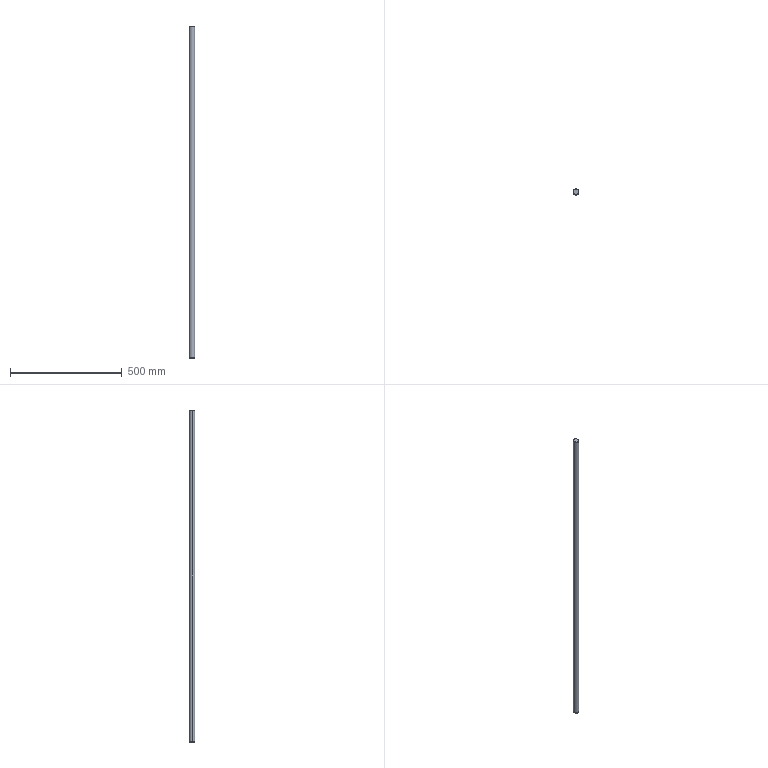Part | SolidWorks | features ICE 3, Extrusion 1, RevCut 1 | 1 solid | 16 faces | box 25 x 25 x 1487 mm | volume 729820 mm3 | cylinder 10 | plane 6 | commonest cylinder face diameters 25 x6 23.9 x4
STEP:
#1=CARTESIAN_POINT('',(-11.95,0.,-30.));
#2=VERTEX_POINT('',#1);
#3=CARTESIAN_POINT('',(11.95,0.,-30.));
#4=VERTEX_POINT('',#3);
#5=CARTESIAN_POINT('',(0.,0.,-30.));
#6=DIRECTION('',(0.,0.,-1.));
#7=DIRECTION('',(-1.,0.,0.));
#8=AXIS2_PLACEMENT_3D('',#5,#6,#7);
#9=CIRCLE('',#8,11.95);
#10=EDGE_CURVE('',#2,#4,#9,.T.);
#11=ORIENTED_EDGE('',*,*,#10,.T.);
#12=CARTESIAN_POINT('',(11.95,0.,-31.3));
#13=VERTEX_POINT('',#12);
#14=CARTESIAN_POINT('',(11.95,0.,1476.033));
#15=DIRECTION('',(0.,0.,-1.));
#16=VECTOR('',#15,1000.);
#17=LINE('',#14,#16);
#18=EDGE_CURVE('',#4,#13,#17,.T.);
#19=ORIENTED_EDGE('',*,*,#18,.T.);
#20=CARTESIAN_POINT('',(-11.95,0.,-31.3));
#21=VERTEX_POINT('',#20);
#22=CARTESIAN_POINT('',(0.,0.,-31.3));
#23=DIRECTION('',(0.,0.,-1.));
#24=DIRECTION('',(-1.,0.,0.));
#25=AXIS2_PLACEMENT_3D('',#22,#23,#24);
#26=CIRCLE('',#25,11.95);
#27=EDGE_CURVE('',#21,#13,#26,.T.);
#28=ORIENTED_EDGE('',*,*,#27,.F.);
#29=CARTESIAN_POINT('',(-11.95,0.,1476.033));
#30=DIRECTION('',(0.,0.,-1.));
#31=VECTOR('',#30,1000.);
#32=LINE('',#29,#31);
#33=EDGE_CURVE('',#2,#21,#32,.T.);
#34=ORIENTED_EDGE('',*,*,#33,.F.);
#35=EDGE_LOOP('',(#11,#19,#28,#34));
#36=FACE_OUTER_BOUND('',#35,.T.);
#37=CARTESIAN_POINT('',(0.,0.,1476.033));
#38=DIRECTION('',(0.,0.,-1.));
#39=DIRECTION('',(-1.,0.,0.));
#40=AXIS2_PLACEMENT_3D('',#37,#38,#39);
#41=CYLINDRICAL_SURFACE('',#40,11.95);
#42=ADVANCED_FACE('',(#36),#41,.T.);
#43=CARTESIAN_POINT('',(-12.5,0.,1450.));
#44=VERTEX_POINT('',#43);
#45=CARTESIAN_POINT('',(12.5,0.,1450.));
#46=VERTEX_POINT('',#45);
#47=CARTESIAN_POINT('',(0.,0.,1450.));
#48=DIRECTION('',(0.,0.,-1.));
#49=DIRECTION('',(-1.,0.,0.));
#50=AXIS2_PLACEMENT_3D('',#47,#48,#49);
#51=CIRCLE('',#50,12.5);
#52=EDGE_CURVE('',#44,#46,#51,.T.);
#53=ORIENTED_EDGE('',*,*,#52,.T.);
#54=CARTESIAN_POINT('',(12.5,0.,-30.));
#55=VERTEX_POINT('',#54);
#56=CARTESIAN_POINT('',(12.5,0.,1470.));
#57=DIRECTION('',(0.,0.,-1.));
#58=VECTOR('',#57,1000.);
#59=LINE('',#56,#58);
#60=EDGE_CURVE('',#46,#55,#59,.T.);
#61=ORIENTED_EDGE('',*,*,#60,.T.);
#62=CARTESIAN_POINT('',(-12.5,0.,-30.));
#63=VERTEX_POINT('',#62);
#64=CARTESIAN_POINT('',(0.,0.,-30.));
#65=DIRECTION('',(0.,0.,-1.));
#66=DIRECTION('',(-1.,0.,0.));
#67=AXIS2_PLACEMENT_3D('',#64,#65,#66);
#68=CIRCLE('',#67,12.5);
#69=EDGE_CURVE('',#63,#55,#68,.T.);
#70=ORIENTED_EDGE('',*,*,#69,.F.);
#71=CARTESIAN_POINT('',(-12.5,0.,1470.));
#72=DIRECTION('',(0.,0.,-1.));
#73=VECTOR('',#72,1000.);
#74=LINE('',#71,#73);
#75=EDGE_CURVE('',#44,#63,#74,.T.);
#76=ORIENTED_EDGE('',*,*,#75,.F.);
#77=EDGE_LOOP('',(#53,#61,#70,#76));
#78=FACE_OUTER_BOUND('',#77,.T.);
#79=CARTESIAN_POINT('',(0.,0.,1470.));
#80=DIRECTION('',(0.,0.,-1.));
#81=DIRECTION('',(-1.,0.,0.));
#82=AXIS2_PLACEMENT_3D('',#79,#80,#81);
#83=CYLINDRICAL_SURFACE('',#82,12.5);
#84=ADVANCED_FACE('',(#78),#83,.T.);
#85=CARTESIAN_POINT('',(-11.95,0.,1451.3));
#86=VERTEX_POINT('',#85);
#87=CARTESIAN_POINT('',(11.95,0.,1451.3));
#88=VERTEX_POINT('',#87);
#89=CARTESIAN_POINT('',(0.,0.,1451.3));
#90=DIRECTION('',(0.,0.,-1.));
#91=DIRECTION('',(-1.,0.,0.));
#92=AXIS2_PLACEMENT_3D('',#89,#90,#91);
#93=CIRCLE('',#92,11.95);
#94=EDGE_CURVE('',#86,#88,#93,.T.);
#95=ORIENTED_EDGE('',*,*,#94,.T.);
#96=CARTESIAN_POINT('',(11.95,0.,1450.));
#97=VERTEX_POINT('',#96);
#98=CARTESIAN_POINT('',(11.95,0.,1476.033));
#99=DIRECTION('',(0.,0.,-1.));
#100=VECTOR('',#99,1000.);
#101=LINE('',#98,#100);
#102=EDGE_CURVE('',#88,#97,#101,.T.);
#103=ORIENTED_EDGE('',*,*,#102,.T.);
#104=CARTESIAN_POINT('',(-11.95,0.,1450.));
#105=VERTEX_POINT('',#104);
#106=CARTESIAN_POINT('',(0.,0.,1450.));
#107=DIRECTION('',(0.,0.,-1.));
#108=DIRECTION('',(-1.,0.,0.));
#109=AXIS2_PLACEMENT_3D('',#106,#107,#108);
#110=CIRCLE('',#109,11.95);
#111=EDGE_CURVE('',#105,#97,#110,.T.);
#112=ORIENTED_EDGE('',*,*,#111,.F.);
#113=CARTESIAN_POINT('',(-11.95,0.,1476.033));
#114=DIRECTION('',(0.,0.,-1.));
#115=VECTOR('',#114,1000.);
#116=LINE('',#113,#115);
#117=EDGE_CURVE('',#86,#105,#116,.T.);
#118=ORIENTED_EDGE('',*,*,#117,.F.);
#119=EDGE_LOOP('',(#95,#103,#112,#118));
#120=FACE_OUTER_BOUND('',#119,.T.);
#121=CARTESIAN_POINT('',(0.,0.,1476.033));
#122=DIRECTION('',(0.,0.,-1.));
#123=DIRECTION('',(-1.,0.,0.));
#124=AXIS2_PLACEMENT_3D('',#121,#122,#123);
#125=CYLINDRICAL_SURFACE('',#124,11.95);
#126=ADVANCED_FACE('',(#120),#125,.T.);
#127=CARTESIAN_POINT('',(12.5,0.,1453.5));
#128=VERTEX_POINT('',#127);
#129=CARTESIAN_POINT('',(-12.5,0.,1453.5));
#130=VERTEX_POINT('',#129);
#131=CARTESIAN_POINT('',(0.,0.,1453.5));
#132=DIRECTION('',(0.,0.,1.));
#133=DIRECTION('',(1.,0.,0.));
#134=AXIS2_PLACEMENT_3D('',#131,#132,#133);
#135=CIRCLE('',#134,12.5);
#136=EDGE_CURVE('',#128,#130,#135,.T.);
#137=ORIENTED_EDGE('',*,*,#136,.F.);
#138=CARTESIAN_POINT('',(12.5,0.,1451.3));
#139=VERTEX_POINT('',#138);
#140=CARTESIAN_POINT('',(12.5,0.,1470.));
#141=DIRECTION('',(0.,0.,-1.));
#142=VECTOR('',#141,1000.);
#143=LINE('',#140,#142);
#144=EDGE_CURVE('',#128,#139,#143,.T.);
#145=ORIENTED_EDGE('',*,*,#144,.T.);
#146=CARTESIAN_POINT('',(-12.5,0.,1451.3));
#147=VERTEX_POINT('',#146);
#148=CARTESIAN_POINT('',(0.,0.,1451.3));
#149=DIRECTION('',(0.,0.,-1.));
#150=DIRECTION('',(-1.,0.,0.));
#151=AXIS2_PLACEMENT_3D('',#148,#149,#150);
#152=CIRCLE('',#151,12.5);
#153=EDGE_CURVE('',#147,#139,#152,.T.);
#154=ORIENTED_EDGE('',*,*,#153,.F.);
#155=CARTESIAN_POINT('',(-12.5,0.,1470.));
#156=DIRECTION('',(0.,0.,-1.));
#157=VECTOR('',#156,1000.);
#158=LINE('',#155,#157);
#159=EDGE_CURVE('',#130,#147,#158,.T.);
#160=ORIENTED_EDGE('',*,*,#159,.F.);
#161=EDGE_LOOP('',(#137,#145,#154,#160));
#162=FACE_OUTER_BOUND('',#161,.T.);
#163=CARTESIAN_POINT('',(0.,0.,1470.));
#164=DIRECTION('',(0.,0.,-1.));
#165=DIRECTION('',(-1.,0.,0.));
#166=AXIS2_PLACEMENT_3D('',#163,#164,#165);
#167=CYLINDRICAL_SURFACE('',#166,12.5);
#168=ADVANCED_FACE('',(#162),#167,.T.);
#169=CARTESIAN_POINT('',(-12.5,0.,-31.3));
#170=VERTEX_POINT('',#169);
#171=CARTESIAN_POINT('',(12.5,0.,-31.3));
#172=VERTEX_POINT('',#171);
#173=CARTESIAN_POINT('',(0.,0.,-31.3));
#174=DIRECTION('',(0.,0.,-1.));
#175=DIRECTION('',(-1.,0.,0.));
#176=AXIS2_PLACEMENT_3D('',#173,#174,#175);
#177=CIRCLE('',#176,12.5);
#178=EDGE_CURVE('',#170,#172,#177,.T.);
#179=ORIENTED_EDGE('',*,*,#178,.T.);
#180=CARTESIAN_POINT('',(12.5,0.,-33.5));
#181=VERTEX_POINT('',#180);
#182=CARTESIAN_POINT('',(12.5,0.,1470.));
#183=DIRECTION('',(0.,0.,-1.));
#184=VECTOR('',#183,1000.);
#185=LINE('',#182,#184);
#186=EDGE_CURVE('',#172,#181,#185,.T.);
#187=ORIENTED_EDGE('',*,*,#186,.T.);
#188=CARTESIAN_POINT('',(-12.5,0.,-33.5));
#189=VERTEX_POINT('',#188);
#190=CARTESIAN_POINT('',(0.,0.,-33.5));
#191=DIRECTION('',(0.,0.,-1.));
#192=DIRECTION('',(-1.,0.,0.));
#193=AXIS2_PLACEMENT_3D('',#190,#191,#192);
#194=CIRCLE('',#193,12.5);
#195=EDGE_CURVE('',#189,#181,#194,.T.);
#196=ORIENTED_EDGE('',*,*,#195,.F.);
#197=CARTESIAN_POINT('',(-12.5,0.,1470.));
#198=DIRECTION('',(0.,0.,-1.));
#199=VECTOR('',#198,1000.);
#200=LINE('',#197,#199);
#201=EDGE_CURVE('',#170,#189,#200,.T.);
#202=ORIENTED_EDGE('',*,*,#201,.F.);
#203=EDGE_LOOP('',(#179,#187,#196,#202));
#204=FACE_OUTER_BOUND('',#203,.T.);
#205=CARTESIAN_POINT('',(0.,0.,1470.));
#206=DIRECTION('',(0.,0.,-1.));
#207=DIRECTION('',(-1.,0.,0.));
#208=AXIS2_PLACEMENT_3D('',#205,#206,#207);
#209=CYLINDRICAL_SURFACE('',#208,12.5);
#210=ADVANCED_FACE('',(#204),#209,.T.);
#211=ORIENTED_EDGE('',*,*,#186,.F.);
#212=CARTESIAN_POINT('',(0.,0.,-31.3));
#213=DIRECTION('',(0.,0.,-1.));
#214=DIRECTION('',(-1.,0.,0.));
#215=AXIS2_PLACEMENT_3D('',#212,#213,#214);
#216=CIRCLE('',#215,12.5);
#217=EDGE_CURVE('',#172,#170,#216,.T.);
#218=ORIENTED_EDGE('',*,*,#217,.T.);
#219=ORIENTED_EDGE('',*,*,#201,.T.);
#220=CARTESIAN_POINT('',(0.,0.,-33.5));
#221=DIRECTION('',(0.,0.,-1.));
#222=DIRECTION('',(-1.,0.,0.));
#223=AXIS2_PLACEMENT_3D('',#220,#221,#222);
#224=CIRCLE('',#223,12.5);
#225=EDGE_CURVE('',#181,#189,#224,.T.);
#226=ORIENTED_EDGE('',*,*,#225,.F.);
#227=EDGE_LOOP('',(#211,#218,#219,#226));
#228=FACE_OUTER_BOUND('',#227,.T.);
#229=CARTESIAN_POINT('',(0.,0.,1470.));
#230=DIRECTION('',(0.,0.,-1.));
#231=DIRECTION('',(-1.,0.,0.));
#232=AXIS2_PLACEMENT_3D('',#229,#230,#231);
#233=CYLINDRICAL_SURFACE('',#232,12.5);
#234=ADVANCED_FACE('',(#228),#233,.T.);
#235=ORIENTED_EDGE('',*,*,#144,.F.);
#236=CARTESIAN_POINT('',(0.,0.,1453.5));
#237=DIRECTION('',(0.,0.,1.));
#238=DIRECTION('',(1.,0.,0.));
#239=AXIS2_PLACEMENT_3D('',#236,#237,#238);
#240=CIRCLE('',#239,12.5);
#241=EDGE_CURVE('',#130,#128,#240,.T.);
#242=ORIENTED_EDGE('',*,*,#241,.F.);
#243=ORIENTED_EDGE('',*,*,#159,.T.);
#244=CARTESIAN_POINT('',(0.,0.,1451.3));
#245=DIRECTION('',(0.,0.,-1.));
#246=DIRECTION('',(-1.,0.,0.));
#247=AXIS2_PLACEMENT_3D('',#244,#245,#246);
#248=CIRCLE('',#247,12.5);
#249=EDGE_CURVE('',#139,#147,#248,.T.);
#250=ORIENTED_EDGE('',*,*,#249,.F.);
#251=EDGE_LOOP('',(#235,#242,#243,#250));
#252=FACE_OUTER_BOUND('',#251,.T.);
#253=CARTESIAN_POINT('',(0.,0.,1470.));
#254=DIRECTION('',(0.,0.,-1.));
#255=DIRECTION('',(-1.,0.,0.));
#256=AXIS2_PLACEMENT_3D('',#253,#254,#255);
#257=CYLINDRICAL_SURFACE('',#256,12.5);
#258=ADVANCED_FACE('',(#252),#257,.T.);
#259=ORIENTED_EDGE('',*,*,#153,.T.);
#260=ORIENTED_EDGE('',*,*,#249,.T.);
#261=EDGE_LOOP('',(#259,#260));
#262=FACE_OUTER_BOUND('',#261,.T.);
#263=ORIENTED_EDGE('',*,*,#94,.F.);
#264=CARTESIAN_POINT('',(0.,0.,1451.3));
#265=DIRECTION('',(0.,0.,-1.));
#266=DIRECTION('',(-1.,0.,0.));
#267=AXIS2_PLACEMENT_3D('',#264,#265,#266);
#268=CIRCLE('',#267,11.95);
#269=EDGE_CURVE('',#88,#86,#268,.T.);
#270=ORIENTED_EDGE('',*,*,#269,.F.);
#271=EDGE_LOOP('',(#263,#270));
#272=FACE_BOUND('',#271,.T.);
#273=CARTESIAN_POINT('',(12.5,0.,1451.3));
#274=DIRECTION('',(0.,0.,-1.));
#275=DIRECTION('',(-1.,0.,0.));
#276=AXIS2_PLACEMENT_3D('',#273,#274,#275);
#277=PLANE('',#276);
#278=ADVANCED_FACE('',(#262,#272),#277,.T.);
#279=ORIENTED_EDGE('',*,*,#102,.F.);
#280=ORIENTED_EDGE('',*,*,#269,.T.);
#281=ORIENTED_EDGE('',*,*,#117,.T.);
#282=CARTESIAN_POINT('',(0.,0.,1450.));
#283=DIRECTION('',(0.,0.,-1.));
#284=DIRECTION('',(-1.,0.,0.));
#285=AXIS2_PLACEMENT_3D('',#282,#283,#284);
#286=CIRCLE('',#285,11.95);
#287=EDGE_CURVE('',#97,#105,#286,.T.);
#288=ORIENTED_EDGE('',*,*,#287,.F.);
#289=EDGE_LOOP('',(#279,#280,#281,#288));
#290=FACE_OUTER_BOUND('',#289,.T.);
#291=CARTESIAN_POINT('',(0.,0.,1476.033));
#292=DIRECTION('',(0.,0.,-1.));
#293=DIRECTION('',(-1.,0.,0.));
#294=AXIS2_PLACEMENT_3D('',#291,#292,#293);
#295=CYLINDRICAL_SURFACE('',#294,11.95);
#296=ADVANCED_FACE('',(#290),#295,.T.);
#297=ORIENTED_EDGE('',*,*,#111,.T.);
#298=ORIENTED_EDGE('',*,*,#287,.T.);
#299=EDGE_LOOP('',(#297,#298));
#300=FACE_BOUND('',#299,.T.);
#301=ORIENTED_EDGE('',*,*,#52,.F.);
#302=CARTESIAN_POINT('',(0.,0.,1450.));
#303=DIRECTION('',(0.,0.,-1.));
#304=DIRECTION('',(-1.,0.,0.));
#305=AXIS2_PLACEMENT_3D('',#302,#303,#304);
#306=CIRCLE('',#305,12.5);
#307=EDGE_CURVE('',#46,#44,#306,.T.);
#308=ORIENTED_EDGE('',*,*,#307,.F.);
#309=EDGE_LOOP('',(#301,#308));
#310=FACE_OUTER_BOUND('',#309,.T.);
#311=CARTESIAN_POINT('',(12.5,0.,1450.));
#312=DIRECTION('',(0.,0.,1.));
#313=DIRECTION('',(1.,0.,0.));
#314=AXIS2_PLACEMENT_3D('',#311,#312,#313);
#315=PLANE('',#314);
#316=ADVANCED_FACE('',(#300,#310),#315,.T.);
#317=ORIENTED_EDGE('',*,*,#60,.F.);
#318=ORIENTED_EDGE('',*,*,#307,.T.);
#319=ORIENTED_EDGE('',*,*,#75,.T.);
#320=CARTESIAN_POINT('',(0.,0.,-30.));
#321=DIRECTION('',(0.,0.,-1.));
#322=DIRECTION('',(-1.,0.,0.));
#323=AXIS2_PLACEMENT_3D('',#320,#321,#322);
#324=CIRCLE('',#323,12.5);
#325=EDGE_CURVE('',#55,#63,#324,.T.);
#326=ORIENTED_EDGE('',*,*,#325,.F.);
#327=EDGE_LOOP('',(#317,#318,#319,#326));
#328=FACE_OUTER_BOUND('',#327,.T.);
#329=CARTESIAN_POINT('',(0.,0.,1470.));
#330=DIRECTION('',(0.,0.,-1.));
#331=DIRECTION('',(-1.,0.,0.));
#332=AXIS2_PLACEMENT_3D('',#329,#330,#331);
#333=CYLINDRICAL_SURFACE('',#332,12.5);
#334=ADVANCED_FACE('',(#328),#333,.T.);
#335=ORIENTED_EDGE('',*,*,#178,.F.);
#336=ORIENTED_EDGE('',*,*,#217,.F.);
#337=EDGE_LOOP('',(#335,#336));
#338=FACE_OUTER_BOUND('',#337,.T.);
#339=ORIENTED_EDGE('',*,*,#27,.T.);
#340=CARTESIAN_POINT('',(0.,0.,-31.3));
#341=DIRECTION('',(0.,0.,-1.));
#342=DIRECTION('',(-1.,0.,0.));
#343=AXIS2_PLACEMENT_3D('',#340,#341,#342);
#344=CIRCLE('',#343,11.95);
#345=EDGE_CURVE('',#13,#21,#344,.T.);
#346=ORIENTED_EDGE('',*,*,#345,.T.);
#347=EDGE_LOOP('',(#339,#346));
#348=FACE_BOUND('',#347,.T.);
#349=CARTESIAN_POINT('',(-12.5,0.,-31.3));
#350=DIRECTION('',(0.,0.,-1.));
#351=DIRECTION('',(-1.,0.,0.));
#352=AXIS2_PLACEMENT_3D('',#349,#350,#351);
#353=PLANE('',#352);
#354=ADVANCED_FACE('',(#338,#348),#353,.F.);
#355=ORIENTED_EDGE('',*,*,#18,.F.);
#356=CARTESIAN_POINT('',(0.,0.,-30.));
#357=DIRECTION('',(0.,0.,-1.));
#358=DIRECTION('',(-1.,0.,0.));
#359=AXIS2_PLACEMENT_3D('',#356,#357,#358);
#360=CIRCLE('',#359,11.95);
#361=EDGE_CURVE('',#4,#2,#360,.T.);
#362=ORIENTED_EDGE('',*,*,#361,.T.);
#363=ORIENTED_EDGE('',*,*,#33,.T.);
#364=ORIENTED_EDGE('',*,*,#345,.F.);
#365=EDGE_LOOP('',(#355,#362,#363,#364));
#366=FACE_OUTER_BOUND('',#365,.T.);
#367=CARTESIAN_POINT('',(0.,0.,1476.033));
#368=DIRECTION('',(0.,0.,-1.));
#369=DIRECTION('',(-1.,0.,0.));
#370=AXIS2_PLACEMENT_3D('',#367,#368,#369);
#371=CYLINDRICAL_SURFACE('',#370,11.95);
#372=ADVANCED_FACE('',(#366),#371,.T.);
#373=ORIENTED_EDGE('',*,*,#10,.F.);
#374=ORIENTED_EDGE('',*,*,#361,.F.);
#375=EDGE_LOOP('',(#373,#374));
#376=FACE_BOUND('',#375,.T.);
#377=ORIENTED_EDGE('',*,*,#69,.T.);
#378=ORIENTED_EDGE('',*,*,#325,.T.);
#379=EDGE_LOOP('',(#377,#378));
#380=FACE_OUTER_BOUND('',#379,.T.);
#381=CARTESIAN_POINT('',(-12.5,0.,-30.));
#382=DIRECTION('',(0.,0.,1.));
#383=DIRECTION('',(1.,0.,0.));
#384=AXIS2_PLACEMENT_3D('',#381,#382,#383);
#385=PLANE('',#384);
#386=ADVANCED_FACE('',(#376,#380),#385,.F.);
#387=ORIENTED_EDGE('',*,*,#241,.T.);
#388=ORIENTED_EDGE('',*,*,#136,.T.);
#389=EDGE_LOOP('',(#387,#388));
#390=FACE_OUTER_BOUND('',#389,.T.);
#391=CARTESIAN_POINT('',(0.,0.,1453.5));
#392=DIRECTION('',(0.,0.,1.));
#393=DIRECTION('',(1.,0.,0.));
#394=AXIS2_PLACEMENT_3D('',#391,#392,#393);
#395=PLANE('',#394);
#396=ADVANCED_FACE('',(#390),#395,.T.);
#397=ORIENTED_EDGE('',*,*,#195,.T.);
#398=ORIENTED_EDGE('',*,*,#225,.T.);
#399=EDGE_LOOP('',(#397,#398));
#400=FACE_OUTER_BOUND('',#399,.T.);
#401=CARTESIAN_POINT('',(0.,0.,-33.5));
#402=DIRECTION('',(0.,0.,-1.));
#403=DIRECTION('',(-1.,0.,0.));
#404=AXIS2_PLACEMENT_3D('',#401,#402,#403);
#405=PLANE('',#404);
#406=ADVANCED_FACE('',(#400),#405,.T.);
#407=CLOSED_SHELL('',(#42,#84,#126,#168,#210,#234,#258,#278,#296,#316,#334,#354,#372,#386,#396,#406));
#408=MANIFOLD_SOLID_BREP('',#407);
#409=CARTESIAN_POINT('',(0.,0.,0.));
#410=DIRECTION('',(0.,0.,1.));
#411=DIRECTION('',(1.,0.,0.));
#412=AXIS2_PLACEMENT_3D('',#409,#410,#411);
#413=(LENGTH_UNIT()NAMED_UNIT(*)SI_UNIT(.MILLI.,.METRE.));
#414=UNCERTAINTY_MEASURE_WITH_UNIT(LENGTH_MEASURE(0.00001),#413,'','');
#415=(NAMED_UNIT(*)PLANE_ANGLE_UNIT()SI_UNIT($,.RADIAN.));
#416=(NAMED_UNIT(*)SI_UNIT($,.STERADIAN.)SOLID_ANGLE_UNIT());
#417=(GEOMETRIC_REPRESENTATION_CONTEXT(3)GLOBAL_UNCERTAINTY_ASSIGNED_CONTEXT((#414))GLOBAL_UNIT_ASSIGNED_CONTEXT((#413,#415,#416))REPRESENTATION_CONTEXT('',''));
#418=ADVANCED_BREP_SHAPE_REPRESENTATION('',(#408,#412),#417);